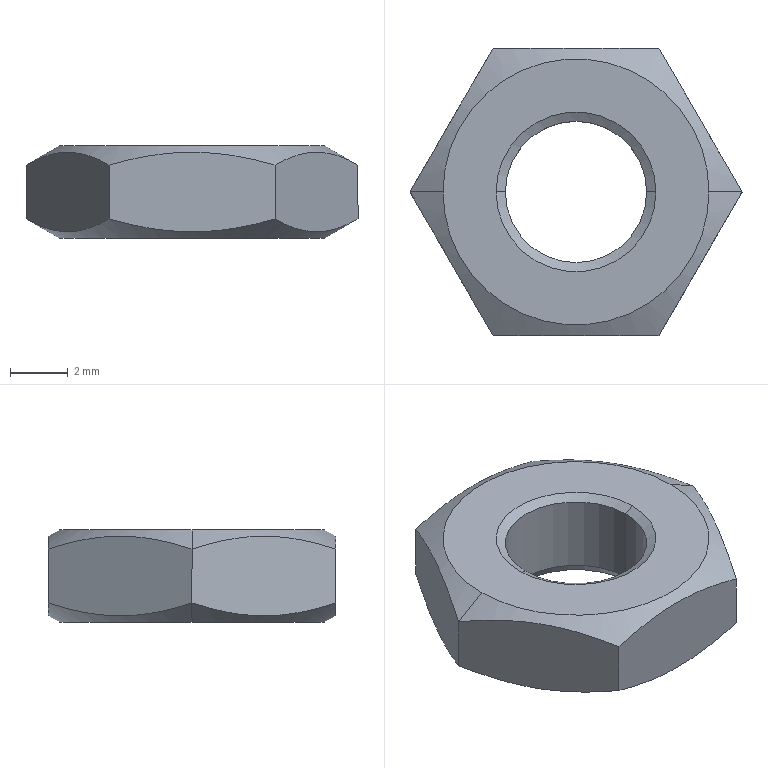Part | SolidWorks | features RevCut 2, Chamfer 1, Extrusion 1, LPattern 1 | 1 solid | 18 faces | box 11.547 x 10 x 3.2 mm | volume 207.259 mm3 | cone 8 | plane 8 | cylinder 2 | commonest cylinder face diameters 4.917 x2
STEP:
#1=CARTESIAN_POINT('',(-2.458,0.,-0.1848));
#2=VERTEX_POINT('',#1);
#3=CARTESIAN_POINT('',(2.458,0.,-0.1848));
#4=VERTEX_POINT('',#3);
#5=CARTESIAN_POINT('',(0.,0.,-0.1848));
#6=DIRECTION('',(0.,0.,1.));
#7=DIRECTION('',(1.,0.,0.));
#8=AXIS2_PLACEMENT_3D('',#5,#6,#7);
#9=CIRCLE('',#8,2.458);
#10=EDGE_CURVE('',#2,#4,#9,.T.);
#11=ORIENTED_EDGE('',*,*,#10,.F.);
#12=CARTESIAN_POINT('',(-2.779,0.,0.));
#13=VERTEX_POINT('',#12);
#14=CARTESIAN_POINT('',(-2.458,0.,-0.1848));
#15=DIRECTION('',(-0.866,0.,0.5));
#16=VECTOR('',#15,1000.);
#17=LINE('',#14,#16);
#18=EDGE_CURVE('',#2,#13,#17,.T.);
#19=ORIENTED_EDGE('',*,*,#18,.T.);
#20=CARTESIAN_POINT('',(2.779,0.,0.));
#21=VERTEX_POINT('',#20);
#22=CARTESIAN_POINT('',(0.,0.,0.));
#23=DIRECTION('',(0.,0.,-1.));
#24=DIRECTION('',(1.,0.,0.));
#25=AXIS2_PLACEMENT_3D('',#22,#23,#24);
#26=CIRCLE('',#25,2.779);
#27=EDGE_CURVE('',#21,#13,#26,.T.);
#28=ORIENTED_EDGE('',*,*,#27,.F.);
#29=CARTESIAN_POINT('',(2.458,0.,-0.1848));
#30=DIRECTION('',(0.866,0.,0.5));
#31=VECTOR('',#30,1000.);
#32=LINE('',#29,#31);
#33=EDGE_CURVE('',#4,#21,#32,.T.);
#34=ORIENTED_EDGE('',*,*,#33,.F.);
#35=EDGE_LOOP('',(#11,#19,#28,#34));
#36=FACE_OUTER_BOUND('',#35,.T.);
#37=CARTESIAN_POINT('',(0.,0.,-0.1848));
#38=DIRECTION('',(0.,0.,1.));
#39=DIRECTION('',(1.,0.,0.));
#40=AXIS2_PLACEMENT_3D('',#37,#38,#39);
#41=CONICAL_SURFACE('',#40,2.458,1.047);
#42=ADVANCED_FACE('',(#36),#41,.F.);
#43=CARTESIAN_POINT('',(2.458,0.,-2.88));
#44=VERTEX_POINT('',#43);
#45=CARTESIAN_POINT('',(-2.458,0.,-2.88));
#46=VERTEX_POINT('',#45);
#47=CARTESIAN_POINT('',(0.,0.,-2.88));
#48=DIRECTION('',(0.,0.,-1.));
#49=DIRECTION('',(1.,0.,0.));
#50=AXIS2_PLACEMENT_3D('',#47,#48,#49);
#51=CIRCLE('',#50,2.458);
#52=EDGE_CURVE('',#44,#46,#51,.T.);
#53=ORIENTED_EDGE('',*,*,#52,.F.);
#54=CARTESIAN_POINT('',(2.643,0.,-3.2));
#55=VERTEX_POINT('',#54);
#56=CARTESIAN_POINT('',(2.643,0.,-3.2));
#57=DIRECTION('',(0.5,0.,-0.866));
#58=VECTOR('',#57,1000.);
#59=LINE('',#56,#58);
#60=EDGE_CURVE('',#44,#55,#59,.T.);
#61=ORIENTED_EDGE('',*,*,#60,.T.);
#62=CARTESIAN_POINT('',(-2.643,0.,-3.2));
#63=VERTEX_POINT('',#62);
#64=CARTESIAN_POINT('',(0.,0.,-3.2));
#65=DIRECTION('',(0.,0.,1.));
#66=DIRECTION('',(1.,0.,0.));
#67=AXIS2_PLACEMENT_3D('',#64,#65,#66);
#68=CIRCLE('',#67,2.643);
#69=EDGE_CURVE('',#63,#55,#68,.T.);
#70=ORIENTED_EDGE('',*,*,#69,.F.);
#71=CARTESIAN_POINT('',(-2.643,0.,-3.2));
#72=DIRECTION('',(-0.5,0.,-0.866));
#73=VECTOR('',#72,1000.);
#74=LINE('',#71,#73);
#75=EDGE_CURVE('',#46,#63,#74,.T.);
#76=ORIENTED_EDGE('',*,*,#75,.F.);
#77=EDGE_LOOP('',(#53,#61,#70,#76));
#78=FACE_OUTER_BOUND('',#77,.T.);
#79=CARTESIAN_POINT('',(0.,0.,-3.2));
#80=DIRECTION('',(0.,0.,-1.));
#81=DIRECTION('',(-1.,0.,0.));
#82=AXIS2_PLACEMENT_3D('',#79,#80,#81);
#83=CONICAL_SURFACE('',#82,2.643,0.5236);
#84=ADVANCED_FACE('',(#78),#83,.F.);
#85=CARTESIAN_POINT('',(-4.625,0.,0.));
#86=VERTEX_POINT('',#85);
#87=CARTESIAN_POINT('',(4.625,0.,0.));
#88=VERTEX_POINT('',#87);
#89=CARTESIAN_POINT('',(0.,0.,0.));
#90=DIRECTION('',(0.,0.,-1.));
#91=DIRECTION('',(-1.,0.,0.));
#92=AXIS2_PLACEMENT_3D('',#89,#90,#91);
#93=CIRCLE('',#92,4.625);
#94=EDGE_CURVE('',#86,#88,#93,.T.);
#95=ORIENTED_EDGE('',*,*,#94,.T.);
#96=CARTESIAN_POINT('',(5.774,0.,-0.6631));
#97=VERTEX_POINT('',#96);
#98=CARTESIAN_POINT('',(4.625,0.,0.));
#99=DIRECTION('',(0.866,0.,-0.5));
#100=VECTOR('',#99,1000.);
#101=LINE('',#98,#100);
#102=EDGE_CURVE('',#88,#97,#101,.T.);
#103=ORIENTED_EDGE('',*,*,#102,.T.);
#104=CARTESIAN_POINT('',(2.887,5.,-0.6631));
#105=VERTEX_POINT('',#104);
#106=CARTESIAN_POINT('',(5.774,0.,-0.6631));
#107=CARTESIAN_POINT('',(5.302,0.8164,-0.391));
#108=CARTESIAN_POINT('',(4.824,1.645,-0.2171));
#109=CARTESIAN_POINT('',(4.21,2.708,-0.2164));
#110=CARTESIAN_POINT('',(4.087,2.921,-0.2268));
#111=CARTESIAN_POINT('',(3.843,3.344,-0.2675));
#112=CARTESIAN_POINT('',(3.722,3.554,-0.2977));
#113=CARTESIAN_POINT('',(3.361,4.179,-0.4144));
#114=CARTESIAN_POINT('',(3.123,4.591,-0.5269));
#115=CARTESIAN_POINT('',(2.887,5.,-0.6631));
#116=B_SPLINE_CURVE_WITH_KNOTS('',3,(#106,#107,#108,#109,#110,#111,#112,#113,#114,#115),.UNSPECIFIED.,.F.,.F.,(4,2,2,2,4),(0.000000238,0.002916,0.003645,0.004373,0.005831),.UNSPECIFIED.);
#117=EDGE_CURVE('',#97,#105,#116,.T.);
#118=ORIENTED_EDGE('',*,*,#117,.T.);
#119=CARTESIAN_POINT('',(-2.887,5.,-0.6631));
#120=VERTEX_POINT('',#119);
#121=CARTESIAN_POINT('',(2.887,5.,-0.6631));
#122=CARTESIAN_POINT('',(2.42,5.,-0.5284));
#123=CARTESIAN_POINT('',(1.947,5.,-0.4162));
#124=CARTESIAN_POINT('',(0.9832,5.,-0.2596));
#125=CARTESIAN_POINT('',(0.4887,5.,-0.2166));
#126=CARTESIAN_POINT('',(-0.487,5.,-0.2165));
#127=CARTESIAN_POINT('',(-0.9718,5.,-0.2584));
#128=CARTESIAN_POINT('',(-1.936,5.,-0.4138));
#129=CARTESIAN_POINT('',(-2.417,5.,-0.5275));
#130=CARTESIAN_POINT('',(-2.887,5.,-0.6631));
#131=B_SPLINE_CURVE_WITH_KNOTS('',3,(#121,#122,#123,#124,#125,#126,#127,#128,#129,#130),.UNSPECIFIED.,.F.,.F.,(4,2,2,2,4),(0.002152,0.003609,0.005066,0.006523,0.007979),.UNSPECIFIED.);
#132=EDGE_CURVE('',#105,#120,#131,.T.);
#133=ORIENTED_EDGE('',*,*,#132,.T.);
#134=CARTESIAN_POINT('',(-5.774,0.,-0.6631));
#135=VERTEX_POINT('',#134);
#136=CARTESIAN_POINT('',(-2.887,5.,-0.6631));
#137=CARTESIAN_POINT('',(-3.358,4.184,-0.391));
#138=CARTESIAN_POINT('',(-3.837,3.355,-0.2171));
#139=CARTESIAN_POINT('',(-4.45,2.292,-0.2164));
#140=CARTESIAN_POINT('',(-4.573,2.079,-0.2268));
#141=CARTESIAN_POINT('',(-4.817,1.656,-0.2675));
#142=CARTESIAN_POINT('',(-4.938,1.446,-0.2977));
#143=CARTESIAN_POINT('',(-5.3,0.8208,-0.4144));
#144=CARTESIAN_POINT('',(-5.538,0.4087,-0.5269));
#145=CARTESIAN_POINT('',(-5.774,0.,-0.6631));
#146=B_SPLINE_CURVE_WITH_KNOTS('',3,(#136,#137,#138,#139,#140,#141,#142,#143,#144,#145),.UNSPECIFIED.,.F.,.F.,(4,2,2,2,4),(0.000000238,0.002916,0.003645,0.004373,0.005831),.UNSPECIFIED.);
#147=EDGE_CURVE('',#120,#135,#146,.T.);
#148=ORIENTED_EDGE('',*,*,#147,.T.);
#149=CARTESIAN_POINT('',(-4.625,0.,0.));
#150=DIRECTION('',(-0.866,0.,-0.5));
#151=VECTOR('',#150,1000.);
#152=LINE('',#149,#151);
#153=EDGE_CURVE('',#86,#135,#152,.T.);
#154=ORIENTED_EDGE('',*,*,#153,.F.);
#155=EDGE_LOOP('',(#95,#103,#118,#133,#148,#154));
#156=FACE_OUTER_BOUND('',#155,.T.);
#157=CARTESIAN_POINT('',(0.,0.,0.));
#158=DIRECTION('',(0.,0.,-1.));
#159=DIRECTION('',(-1.,0.,0.));
#160=AXIS2_PLACEMENT_3D('',#157,#158,#159);
#161=CONICAL_SURFACE('',#160,4.625,1.047);
#162=ADVANCED_FACE('',(#156),#161,.T.);
#163=CARTESIAN_POINT('',(-4.625,0.,-3.2));
#164=VERTEX_POINT('',#163);
#165=CARTESIAN_POINT('',(4.625,0.,-3.2));
#166=VERTEX_POINT('',#165);
#167=CARTESIAN_POINT('',(0.,0.,-3.2));
#168=DIRECTION('',(0.,0.,-1.));
#169=DIRECTION('',(-1.,0.,0.));
#170=AXIS2_PLACEMENT_3D('',#167,#168,#169);
#171=CIRCLE('',#170,4.625);
#172=EDGE_CURVE('',#164,#166,#171,.T.);
#173=ORIENTED_EDGE('',*,*,#172,.F.);
#174=CARTESIAN_POINT('',(-5.774,0.,-2.537));
#175=VERTEX_POINT('',#174);
#176=CARTESIAN_POINT('',(-5.774,0.,-2.537));
#177=DIRECTION('',(-0.866,0.,0.5));
#178=VECTOR('',#177,1000.);
#179=LINE('',#176,#178);
#180=EDGE_CURVE('',#164,#175,#179,.T.);
#181=ORIENTED_EDGE('',*,*,#180,.T.);
#182=CARTESIAN_POINT('',(-2.887,5.,-2.537));
#183=VERTEX_POINT('',#182);
#184=CARTESIAN_POINT('',(-5.774,0.,-2.537));
#185=CARTESIAN_POINT('',(-5.302,0.8164,-2.809));
#186=CARTESIAN_POINT('',(-4.824,1.645,-2.983));
#187=CARTESIAN_POINT('',(-4.21,2.708,-2.984));
#188=CARTESIAN_POINT('',(-4.087,2.921,-2.973));
#189=CARTESIAN_POINT('',(-3.843,3.344,-2.933));
#190=CARTESIAN_POINT('',(-3.722,3.554,-2.902));
#191=CARTESIAN_POINT('',(-3.361,4.179,-2.786));
#192=CARTESIAN_POINT('',(-3.123,4.591,-2.673));
#193=CARTESIAN_POINT('',(-2.887,5.,-2.537));
#194=B_SPLINE_CURVE_WITH_KNOTS('',3,(#184,#185,#186,#187,#188,#189,#190,#191,#192,#193),.UNSPECIFIED.,.F.,.F.,(4,2,2,2,4),(0.000000238,0.002916,0.003645,0.004373,0.005831),.UNSPECIFIED.);
#195=EDGE_CURVE('',#175,#183,#194,.T.);
#196=ORIENTED_EDGE('',*,*,#195,.T.);
#197=CARTESIAN_POINT('',(2.887,5.,-2.537));
#198=VERTEX_POINT('',#197);
#199=CARTESIAN_POINT('',(-2.887,5.,-2.537));
#200=CARTESIAN_POINT('',(-2.417,5.,-2.672));
#201=CARTESIAN_POINT('',(-1.936,5.,-2.786));
#202=CARTESIAN_POINT('',(-0.9718,5.,-2.942));
#203=CARTESIAN_POINT('',(-0.487,5.,-2.984));
#204=CARTESIAN_POINT('',(0.4887,5.,-2.983));
#205=CARTESIAN_POINT('',(0.9832,5.,-2.94));
#206=CARTESIAN_POINT('',(1.947,5.,-2.784));
#207=CARTESIAN_POINT('',(2.42,5.,-2.672));
#208=CARTESIAN_POINT('',(2.887,5.,-2.537));
#209=B_SPLINE_CURVE_WITH_KNOTS('',3,(#199,#200,#201,#202,#203,#204,#205,#206,#207,#208),.UNSPECIFIED.,.F.,.F.,(4,2,2,2,4),(0.005117,0.006577,0.008038,0.009498,0.01096),.UNSPECIFIED.);
#210=EDGE_CURVE('',#183,#198,#209,.T.);
#211=ORIENTED_EDGE('',*,*,#210,.T.);
#212=CARTESIAN_POINT('',(5.774,0.,-2.537));
#213=VERTEX_POINT('',#212);
#214=CARTESIAN_POINT('',(2.887,5.,-2.537));
#215=CARTESIAN_POINT('',(3.358,4.184,-2.809));
#216=CARTESIAN_POINT('',(3.837,3.355,-2.983));
#217=CARTESIAN_POINT('',(4.45,2.292,-2.984));
#218=CARTESIAN_POINT('',(4.573,2.079,-2.973));
#219=CARTESIAN_POINT('',(4.817,1.656,-2.933));
#220=CARTESIAN_POINT('',(4.938,1.446,-2.902));
#221=CARTESIAN_POINT('',(5.3,0.8208,-2.786));
#222=CARTESIAN_POINT('',(5.538,0.4087,-2.673));
#223=CARTESIAN_POINT('',(5.774,0.,-2.537));
#224=B_SPLINE_CURVE_WITH_KNOTS('',3,(#214,#215,#216,#217,#218,#219,#220,#221,#222,#223),.UNSPECIFIED.,.F.,.F.,(4,2,2,2,4),(0.000000238,0.002916,0.003645,0.004373,0.005831),.UNSPECIFIED.);
#225=EDGE_CURVE('',#198,#213,#224,.T.);
#226=ORIENTED_EDGE('',*,*,#225,.T.);
#227=CARTESIAN_POINT('',(5.774,0.,-2.537));
#228=DIRECTION('',(0.866,0.,0.5));
#229=VECTOR('',#228,1000.);
#230=LINE('',#227,#229);
#231=EDGE_CURVE('',#166,#213,#230,.T.);
#232=ORIENTED_EDGE('',*,*,#231,.F.);
#233=EDGE_LOOP('',(#173,#181,#196,#211,#226,#232));
#234=FACE_OUTER_BOUND('',#233,.T.);
#235=CARTESIAN_POINT('',(0.,0.,-2.537));
#236=DIRECTION('',(0.,0.,1.));
#237=DIRECTION('',(1.,0.,0.));
#238=AXIS2_PLACEMENT_3D('',#235,#236,#237);
#239=CONICAL_SURFACE('',#238,5.774,1.047);
#240=ADVANCED_FACE('',(#234),#239,.T.);
#241=ORIENTED_EDGE('',*,*,#52,.T.);
#242=CARTESIAN_POINT('',(-2.458,0.,-3.2));
#243=DIRECTION('',(0.,0.,1.));
#244=VECTOR('',#243,1000.);
#245=LINE('',#242,#244);
#246=EDGE_CURVE('',#46,#2,#245,.T.);
#247=ORIENTED_EDGE('',*,*,#246,.T.);
#248=ORIENTED_EDGE('',*,*,#10,.T.);
#249=CARTESIAN_POINT('',(2.458,0.,-3.2));
#250=DIRECTION('',(0.,0.,1.));
#251=VECTOR('',#250,1000.);
#252=LINE('',#249,#251);
#253=EDGE_CURVE('',#44,#4,#252,.T.);
#254=ORIENTED_EDGE('',*,*,#253,.F.);
#255=EDGE_LOOP('',(#241,#247,#248,#254));
#256=FACE_OUTER_BOUND('',#255,.T.);
#257=CARTESIAN_POINT('',(0.,0.,-3.2));
#258=DIRECTION('',(0.,0.,1.));
#259=DIRECTION('',(1.,0.,0.));
#260=AXIS2_PLACEMENT_3D('',#257,#258,#259);
#261=CYLINDRICAL_SURFACE('',#260,2.458);
#262=ADVANCED_FACE('',(#256),#261,.F.);
#263=CARTESIAN_POINT('',(-2.887,-5.,-0.6631));
#264=VERTEX_POINT('',#263);
#265=CARTESIAN_POINT('',(2.887,-5.,-0.6631));
#266=VERTEX_POINT('',#265);
#267=CARTESIAN_POINT('',(-2.887,-5.,-0.6631));
#268=CARTESIAN_POINT('',(-2.417,-5.,-0.5275));
#269=CARTESIAN_POINT('',(-1.936,-5.,-0.4138));
#270=CARTESIAN_POINT('',(-0.9718,-5.,-0.2584));
#271=CARTESIAN_POINT('',(-0.487,-5.,-0.2165));
#272=CARTESIAN_POINT('',(0.4887,-5.,-0.2166));
#273=CARTESIAN_POINT('',(0.9832,-5.,-0.2596));
#274=CARTESIAN_POINT('',(1.947,-5.,-0.4162));
#275=CARTESIAN_POINT('',(2.42,-5.,-0.5284));
#276=CARTESIAN_POINT('',(2.887,-5.,-0.6631));
#277=B_SPLINE_CURVE_WITH_KNOTS('',3,(#267,#268,#269,#270,#271,#272,#273,#274,#275,#276),.UNSPECIFIED.,.F.,.F.,(4,2,2,2,4),(0.005117,0.006577,0.008038,0.009498,0.01096),.UNSPECIFIED.);
#278=EDGE_CURVE('',#264,#266,#277,.T.);
#279=ORIENTED_EDGE('',*,*,#278,.F.);
#280=CARTESIAN_POINT('',(-2.887,-5.,-2.537));
#281=VERTEX_POINT('',#280);
#282=CARTESIAN_POINT('',(-2.887,-5.,-3.2));
#283=DIRECTION('',(0.,0.,1.));
#284=VECTOR('',#283,1000.);
#285=LINE('',#282,#284);
#286=EDGE_CURVE('',#281,#264,#285,.T.);
#287=ORIENTED_EDGE('',*,*,#286,.F.);
#288=CARTESIAN_POINT('',(2.887,-5.,-2.537));
#289=VERTEX_POINT('',#288);
#290=CARTESIAN_POINT('',(2.887,-5.,-2.537));
#291=CARTESIAN_POINT('',(2.42,-5.,-2.672));
#292=CARTESIAN_POINT('',(1.947,-5.,-2.784));
#293=CARTESIAN_POINT('',(0.9832,-5.,-2.94));
#294=CARTESIAN_POINT('',(0.4887,-5.,-2.983));
#295=CARTESIAN_POINT('',(-0.487,-5.,-2.984));
#296=CARTESIAN_POINT('',(-0.9718,-5.,-2.942));
#297=CARTESIAN_POINT('',(-1.936,-5.,-2.786));
#298=CARTESIAN_POINT('',(-2.417,-5.,-2.672));
#299=CARTESIAN_POINT('',(-2.887,-5.,-2.537));
#300=B_SPLINE_CURVE_WITH_KNOTS('',3,(#290,#291,#292,#293,#294,#295,#296,#297,#298,#299),.UNSPECIFIED.,.F.,.F.,(4,2,2,2,4),(0.002152,0.003609,0.005066,0.006523,0.007979),.UNSPECIFIED.);
#301=EDGE_CURVE('',#289,#281,#300,.T.);
#302=ORIENTED_EDGE('',*,*,#301,.F.);
#303=CARTESIAN_POINT('',(2.887,-5.,-3.2));
#304=DIRECTION('',(0.,0.,1.));
#305=VECTOR('',#304,1000.);
#306=LINE('',#303,#305);
#307=EDGE_CURVE('',#289,#266,#306,.T.);
#308=ORIENTED_EDGE('',*,*,#307,.T.);
#309=EDGE_LOOP('',(#279,#287,#302,#308));
#310=FACE_OUTER_BOUND('',#309,.T.);
#311=CARTESIAN_POINT('',(-2.887,-5.,-3.2));
#312=DIRECTION('',(0.,-1.,0.));
#313=DIRECTION('',(1.,0.,0.));
#314=AXIS2_PLACEMENT_3D('',#311,#312,#313);
#315=PLANE('',#314);
#316=ADVANCED_FACE('',(#310),#315,.T.);
#317=CARTESIAN_POINT('',(-5.774,0.,-0.6631));
#318=CARTESIAN_POINT('',(-5.302,-0.8164,-0.391));
#319=CARTESIAN_POINT('',(-4.824,-1.645,-0.2171));
#320=CARTESIAN_POINT('',(-4.21,-2.708,-0.2164));
#321=CARTESIAN_POINT('',(-4.087,-2.921,-0.2268));
#322=CARTESIAN_POINT('',(-3.843,-3.344,-0.2675));
#323=CARTESIAN_POINT('',(-3.722,-3.554,-0.2977));
#324=CARTESIAN_POINT('',(-3.361,-4.179,-0.4144));
#325=CARTESIAN_POINT('',(-3.123,-4.591,-0.5269));
#326=CARTESIAN_POINT('',(-2.887,-5.,-0.6631));
#327=B_SPLINE_CURVE_WITH_KNOTS('',3,(#317,#318,#319,#320,#321,#322,#323,#324,#325,#326),.UNSPECIFIED.,.F.,.F.,(4,2,2,2,4),(0.000000238,0.002916,0.003645,0.004373,0.005831),.UNSPECIFIED.);
#328=EDGE_CURVE('',#135,#264,#327,.T.);
#329=ORIENTED_EDGE('',*,*,#328,.F.);
#330=CARTESIAN_POINT('',(-5.774,0.,-3.2));
#331=DIRECTION('',(0.,0.,1.));
#332=VECTOR('',#331,1000.);
#333=LINE('',#330,#332);
#334=EDGE_CURVE('',#175,#135,#333,.T.);
#335=ORIENTED_EDGE('',*,*,#334,.F.);
#336=CARTESIAN_POINT('',(-2.887,-5.,-2.537));
#337=CARTESIAN_POINT('',(-3.358,-4.184,-2.809));
#338=CARTESIAN_POINT('',(-3.837,-3.355,-2.983));
#339=CARTESIAN_POINT('',(-4.45,-2.292,-2.984));
#340=CARTESIAN_POINT('',(-4.573,-2.079,-2.973));
#341=CARTESIAN_POINT('',(-4.817,-1.656,-2.933));
#342=CARTESIAN_POINT('',(-4.938,-1.446,-2.902));
#343=CARTESIAN_POINT('',(-5.3,-0.8208,-2.786));
#344=CARTESIAN_POINT('',(-5.538,-0.4087,-2.673));
#345=CARTESIAN_POINT('',(-5.774,0.,-2.537));
#346=B_SPLINE_CURVE_WITH_KNOTS('',3,(#336,#337,#338,#339,#340,#341,#342,#343,#344,#345),.UNSPECIFIED.,.F.,.F.,(4,2,2,2,4),(0.000000238,0.002916,0.003645,0.004373,0.005831),.UNSPECIFIED.);
#347=EDGE_CURVE('',#281,#175,#346,.T.);
#348=ORIENTED_EDGE('',*,*,#347,.F.);
#349=ORIENTED_EDGE('',*,*,#286,.T.);
#350=EDGE_LOOP('',(#329,#335,#348,#349));
#351=FACE_OUTER_BOUND('',#350,.T.);
#352=CARTESIAN_POINT('',(-5.774,0.,-3.2));
#353=DIRECTION('',(-0.866,-0.5,0.));
#354=DIRECTION('',(0.5,-0.866,0.));
#355=AXIS2_PLACEMENT_3D('',#352,#353,#354);
#356=PLANE('',#355);
#357=ADVANCED_FACE('',(#351),#356,.T.);
#358=ORIENTED_EDGE('',*,*,#147,.F.);
#359=CARTESIAN_POINT('',(-2.887,5.,-3.2));
#360=DIRECTION('',(0.,0.,1.));
#361=VECTOR('',#360,1000.);
#362=LINE('',#359,#361);
#363=EDGE_CURVE('',#183,#120,#362,.T.);
#364=ORIENTED_EDGE('',*,*,#363,.F.);
#365=ORIENTED_EDGE('',*,*,#195,.F.);
#366=ORIENTED_EDGE('',*,*,#334,.T.);
#367=EDGE_LOOP('',(#358,#364,#365,#366));
#368=FACE_OUTER_BOUND('',#367,.T.);
#369=CARTESIAN_POINT('',(-2.887,5.,-3.2));
#370=DIRECTION('',(-0.866,0.5,0.));
#371=DIRECTION('',(-0.5,-0.866,0.));
#372=AXIS2_PLACEMENT_3D('',#369,#370,#371);
#373=PLANE('',#372);
#374=ADVANCED_FACE('',(#368),#373,.T.);
#375=ORIENTED_EDGE('',*,*,#132,.F.);
#376=CARTESIAN_POINT('',(2.887,5.,-3.2));
#377=DIRECTION('',(0.,0.,1.));
#378=VECTOR('',#377,1000.);
#379=LINE('',#376,#378);
#380=EDGE_CURVE('',#198,#105,#379,.T.);
#381=ORIENTED_EDGE('',*,*,#380,.F.);
#382=ORIENTED_EDGE('',*,*,#210,.F.);
#383=ORIENTED_EDGE('',*,*,#363,.T.);
#384=EDGE_LOOP('',(#375,#381,#382,#383));
#385=FACE_OUTER_BOUND('',#384,.T.);
#386=CARTESIAN_POINT('',(2.887,5.,-3.2));
#387=DIRECTION('',(0.,1.,0.));
#388=DIRECTION('',(-1.,0.,0.));
#389=AXIS2_PLACEMENT_3D('',#386,#387,#388);
#390=PLANE('',#389);
#391=ADVANCED_FACE('',(#385),#390,.T.);
#392=ORIENTED_EDGE('',*,*,#117,.F.);
#393=CARTESIAN_POINT('',(5.774,0.,-3.2));
#394=DIRECTION('',(0.,0.,1.));
#395=VECTOR('',#394,1000.);
#396=LINE('',#393,#395);
#397=EDGE_CURVE('',#213,#97,#396,.T.);
#398=ORIENTED_EDGE('',*,*,#397,.F.);
#399=ORIENTED_EDGE('',*,*,#225,.F.);
#400=ORIENTED_EDGE('',*,*,#380,.T.);
#401=EDGE_LOOP('',(#392,#398,#399,#400));
#402=FACE_OUTER_BOUND('',#401,.T.);
#403=CARTESIAN_POINT('',(5.774,0.,-3.2));
#404=DIRECTION('',(0.866,0.5,0.));
#405=DIRECTION('',(-0.5,0.866,0.));
#406=AXIS2_PLACEMENT_3D('',#403,#404,#405);
#407=PLANE('',#406);
#408=ADVANCED_FACE('',(#402),#407,.T.);
#409=CARTESIAN_POINT('',(2.887,-5.,-0.6631));
#410=CARTESIAN_POINT('',(3.358,-4.184,-0.391));
#411=CARTESIAN_POINT('',(3.837,-3.355,-0.2171));
#412=CARTESIAN_POINT('',(4.45,-2.292,-0.2164));
#413=CARTESIAN_POINT('',(4.573,-2.079,-0.2268));
#414=CARTESIAN_POINT('',(4.817,-1.656,-0.2675));
#415=CARTESIAN_POINT('',(4.938,-1.446,-0.2977));
#416=CARTESIAN_POINT('',(5.3,-0.8208,-0.4144));
#417=CARTESIAN_POINT('',(5.538,-0.4087,-0.5269));
#418=CARTESIAN_POINT('',(5.774,0.,-0.6631));
#419=B_SPLINE_CURVE_WITH_KNOTS('',3,(#409,#410,#411,#412,#413,#414,#415,#416,#417,#418),.UNSPECIFIED.,.F.,.F.,(4,2,2,2,4),(0.000000238,0.002916,0.003645,0.004373,0.005831),.UNSPECIFIED.);
#420=EDGE_CURVE('',#266,#97,#419,.T.);
#421=ORIENTED_EDGE('',*,*,#420,.F.);
#422=ORIENTED_EDGE('',*,*,#307,.F.);
#423=CARTESIAN_POINT('',(5.774,0.,-2.537));
#424=CARTESIAN_POINT('',(5.302,-0.8164,-2.809));
#425=CARTESIAN_POINT('',(4.824,-1.645,-2.983));
#426=CARTESIAN_POINT('',(4.21,-2.708,-2.984));
#427=CARTESIAN_POINT('',(4.087,-2.921,-2.973));
#428=CARTESIAN_POINT('',(3.843,-3.344,-2.933));
#429=CARTESIAN_POINT('',(3.722,-3.554,-2.902));
#430=CARTESIAN_POINT('',(3.361,-4.179,-2.786));
#431=CARTESIAN_POINT('',(3.123,-4.591,-2.673));
#432=CARTESIAN_POINT('',(2.887,-5.,-2.537));
#433=B_SPLINE_CURVE_WITH_KNOTS('',3,(#423,#424,#425,#426,#427,#428,#429,#430,#431,#432),.UNSPECIFIED.,.F.,.F.,(4,2,2,2,4),(0.000000238,0.002916,0.003645,0.004373,0.005831),.UNSPECIFIED.);
#434=EDGE_CURVE('',#213,#289,#433,.T.);
#435=ORIENTED_EDGE('',*,*,#434,.F.);
#436=ORIENTED_EDGE('',*,*,#397,.T.);
#437=EDGE_LOOP('',(#421,#422,#435,#436));
#438=FACE_OUTER_BOUND('',#437,.T.);
#439=CARTESIAN_POINT('',(2.887,-5.,-3.2));
#440=DIRECTION('',(0.866,-0.5,0.));
#441=DIRECTION('',(0.5,0.866,0.));
#442=AXIS2_PLACEMENT_3D('',#439,#440,#441);
#443=PLANE('',#442);
#444=ADVANCED_FACE('',(#438),#443,.T.);
#445=ORIENTED_EDGE('',*,*,#69,.T.);
#446=CARTESIAN_POINT('',(0.,0.,-3.2));
#447=DIRECTION('',(0.,0.,1.));
#448=DIRECTION('',(1.,0.,0.));
#449=AXIS2_PLACEMENT_3D('',#446,#447,#448);
#450=CIRCLE('',#449,2.643);
#451=EDGE_CURVE('',#55,#63,#450,.T.);
#452=ORIENTED_EDGE('',*,*,#451,.T.);
#453=EDGE_LOOP('',(#445,#452));
#454=FACE_BOUND('',#453,.T.);
#455=CARTESIAN_POINT('',(0.,0.,-3.2));
#456=DIRECTION('',(0.,0.,-1.));
#457=DIRECTION('',(-1.,0.,0.));
#458=AXIS2_PLACEMENT_3D('',#455,#456,#457);
#459=CIRCLE('',#458,4.625);
#460=EDGE_CURVE('',#166,#164,#459,.T.);
#461=ORIENTED_EDGE('',*,*,#460,.T.);
#462=ORIENTED_EDGE('',*,*,#172,.T.);
#463=EDGE_LOOP('',(#461,#462));
#464=FACE_OUTER_BOUND('',#463,.T.);
#465=CARTESIAN_POINT('',(2.887,-5.,-3.2));
#466=DIRECTION('',(0.,0.,1.));
#467=DIRECTION('',(1.,0.,0.));
#468=AXIS2_PLACEMENT_3D('',#465,#466,#467);
#469=PLANE('',#468);
#470=ADVANCED_FACE('',(#454,#464),#469,.F.);
#471=ORIENTED_EDGE('',*,*,#27,.T.);
#472=CARTESIAN_POINT('',(0.,0.,0.));
#473=DIRECTION('',(0.,0.,-1.));
#474=DIRECTION('',(1.,0.,0.));
#475=AXIS2_PLACEMENT_3D('',#472,#473,#474);
#476=CIRCLE('',#475,2.779);
#477=EDGE_CURVE('',#13,#21,#476,.T.);
#478=ORIENTED_EDGE('',*,*,#477,.T.);
#479=EDGE_LOOP('',(#471,#478));
#480=FACE_BOUND('',#479,.T.);
#481=ORIENTED_EDGE('',*,*,#94,.F.);
#482=CARTESIAN_POINT('',(0.,0.,0.));
#483=DIRECTION('',(0.,0.,-1.));
#484=DIRECTION('',(-1.,0.,0.));
#485=AXIS2_PLACEMENT_3D('',#482,#483,#484);
#486=CIRCLE('',#485,4.625);
#487=EDGE_CURVE('',#88,#86,#486,.T.);
#488=ORIENTED_EDGE('',*,*,#487,.F.);
#489=EDGE_LOOP('',(#481,#488));
#490=FACE_OUTER_BOUND('',#489,.T.);
#491=CARTESIAN_POINT('',(2.887,-5.,0.));
#492=DIRECTION('',(0.,0.,1.));
#493=DIRECTION('',(1.,0.,0.));
#494=AXIS2_PLACEMENT_3D('',#491,#492,#493);
#495=PLANE('',#494);
#496=ADVANCED_FACE('',(#480,#490),#495,.T.);
#497=ORIENTED_EDGE('',*,*,#246,.F.);
#498=CARTESIAN_POINT('',(0.,0.,-2.88));
#499=DIRECTION('',(0.,0.,-1.));
#500=DIRECTION('',(1.,0.,0.));
#501=AXIS2_PLACEMENT_3D('',#498,#499,#500);
#502=CIRCLE('',#501,2.458);
#503=EDGE_CURVE('',#46,#44,#502,.T.);
#504=ORIENTED_EDGE('',*,*,#503,.T.);
#505=ORIENTED_EDGE('',*,*,#253,.T.);
#506=CARTESIAN_POINT('',(0.,0.,-0.1848));
#507=DIRECTION('',(0.,0.,1.));
#508=DIRECTION('',(1.,0.,0.));
#509=AXIS2_PLACEMENT_3D('',#506,#507,#508);
#510=CIRCLE('',#509,2.458);
#511=EDGE_CURVE('',#4,#2,#510,.T.);
#512=ORIENTED_EDGE('',*,*,#511,.T.);
#513=EDGE_LOOP('',(#497,#504,#505,#512));
#514=FACE_OUTER_BOUND('',#513,.T.);
#515=CARTESIAN_POINT('',(0.,0.,-3.2));
#516=DIRECTION('',(0.,0.,1.));
#517=DIRECTION('',(1.,0.,0.));
#518=AXIS2_PLACEMENT_3D('',#515,#516,#517);
#519=CYLINDRICAL_SURFACE('',#518,2.458);
#520=ADVANCED_FACE('',(#514),#519,.F.);
#521=ORIENTED_EDGE('',*,*,#180,.F.);
#522=ORIENTED_EDGE('',*,*,#460,.F.);
#523=ORIENTED_EDGE('',*,*,#231,.T.);
#524=ORIENTED_EDGE('',*,*,#434,.T.);
#525=ORIENTED_EDGE('',*,*,#301,.T.);
#526=ORIENTED_EDGE('',*,*,#347,.T.);
#527=EDGE_LOOP('',(#521,#522,#523,#524,#525,#526));
#528=FACE_OUTER_BOUND('',#527,.T.);
#529=CARTESIAN_POINT('',(0.,0.,-2.537));
#530=DIRECTION('',(0.,0.,1.));
#531=DIRECTION('',(1.,0.,0.));
#532=AXIS2_PLACEMENT_3D('',#529,#530,#531);
#533=CONICAL_SURFACE('',#532,5.774,1.047);
#534=ADVANCED_FACE('',(#528),#533,.T.);
#535=ORIENTED_EDGE('',*,*,#102,.F.);
#536=ORIENTED_EDGE('',*,*,#487,.T.);
#537=ORIENTED_EDGE('',*,*,#153,.T.);
#538=ORIENTED_EDGE('',*,*,#328,.T.);
#539=ORIENTED_EDGE('',*,*,#278,.T.);
#540=ORIENTED_EDGE('',*,*,#420,.T.);
#541=EDGE_LOOP('',(#535,#536,#537,#538,#539,#540));
#542=FACE_OUTER_BOUND('',#541,.T.);
#543=CARTESIAN_POINT('',(0.,0.,0.));
#544=DIRECTION('',(0.,0.,-1.));
#545=DIRECTION('',(-1.,0.,0.));
#546=AXIS2_PLACEMENT_3D('',#543,#544,#545);
#547=CONICAL_SURFACE('',#546,4.625,1.047);
#548=ADVANCED_FACE('',(#542),#547,.T.);
#549=ORIENTED_EDGE('',*,*,#60,.F.);
#550=ORIENTED_EDGE('',*,*,#503,.F.);
#551=ORIENTED_EDGE('',*,*,#75,.T.);
#552=ORIENTED_EDGE('',*,*,#451,.F.);
#553=EDGE_LOOP('',(#549,#550,#551,#552));
#554=FACE_OUTER_BOUND('',#553,.T.);
#555=CARTESIAN_POINT('',(0.,0.,-3.2));
#556=DIRECTION('',(0.,0.,-1.));
#557=DIRECTION('',(-1.,0.,0.));
#558=AXIS2_PLACEMENT_3D('',#555,#556,#557);
#559=CONICAL_SURFACE('',#558,2.643,0.5236);
#560=ADVANCED_FACE('',(#554),#559,.F.);
#561=ORIENTED_EDGE('',*,*,#18,.F.);
#562=ORIENTED_EDGE('',*,*,#511,.F.);
#563=ORIENTED_EDGE('',*,*,#33,.T.);
#564=ORIENTED_EDGE('',*,*,#477,.F.);
#565=EDGE_LOOP('',(#561,#562,#563,#564));
#566=FACE_OUTER_BOUND('',#565,.T.);
#567=CARTESIAN_POINT('',(0.,0.,-0.1848));
#568=DIRECTION('',(0.,0.,1.));
#569=DIRECTION('',(1.,0.,0.));
#570=AXIS2_PLACEMENT_3D('',#567,#568,#569);
#571=CONICAL_SURFACE('',#570,2.458,1.047);
#572=ADVANCED_FACE('',(#566),#571,.F.);
#573=CLOSED_SHELL('',(#42,#84,#162,#240,#262,#316,#357,#374,#391,#408,#444,#470,#496,#520,#534,#548,#560,#572));
#574=MANIFOLD_SOLID_BREP('',#573);
#575=CARTESIAN_POINT('',(0.,0.,0.));
#576=DIRECTION('',(0.,0.,1.));
#577=DIRECTION('',(1.,0.,0.));
#578=AXIS2_PLACEMENT_3D('',#575,#576,#577);
#579=(LENGTH_UNIT()NAMED_UNIT(*)SI_UNIT(.MILLI.,.METRE.));
#580=UNCERTAINTY_MEASURE_WITH_UNIT(LENGTH_MEASURE(0.00001),#579,'','');
#581=(NAMED_UNIT(*)PLANE_ANGLE_UNIT()SI_UNIT($,.RADIAN.));
#582=(NAMED_UNIT(*)SI_UNIT($,.STERADIAN.)SOLID_ANGLE_UNIT());
#583=(GEOMETRIC_REPRESENTATION_CONTEXT(3)GLOBAL_UNCERTAINTY_ASSIGNED_CONTEXT((#580))GLOBAL_UNIT_ASSIGNED_CONTEXT((#579,#581,#582))REPRESENTATION_CONTEXT('',''));
#584=ADVANCED_BREP_SHAPE_REPRESENTATION('',(#574,#578),#583);